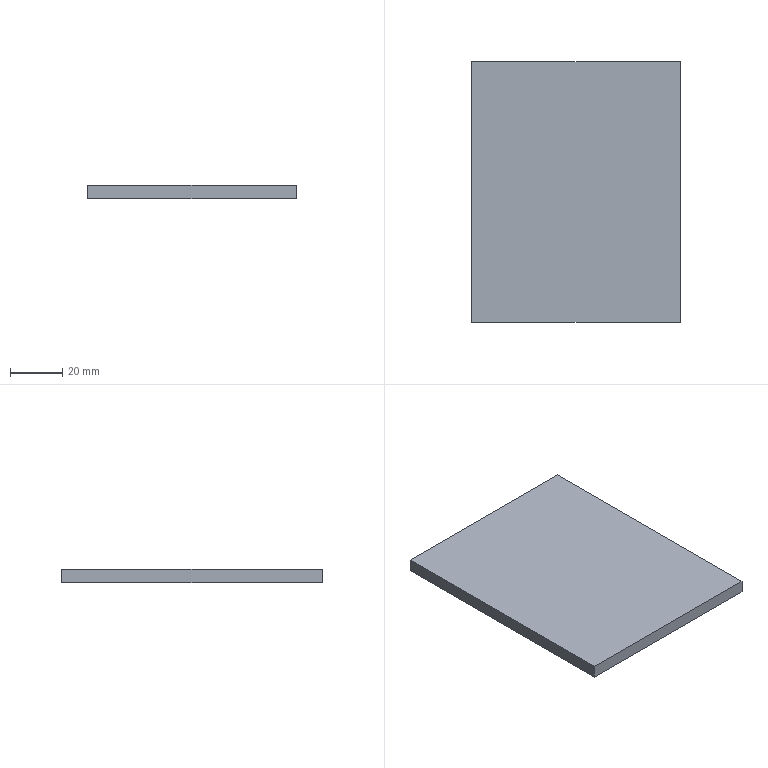Part | STEP file | MYT-A01-P41 | 1 solid | 6 faces | box 80 x 100 x 5 mm | volume 40000 mm3 | plane 6
STEP:
#1=CARTESIAN_POINT('',(40.,-50.,0.));
#2=VERTEX_POINT('',#1);
#3=CARTESIAN_POINT('',(40.,50.,0.));
#4=VERTEX_POINT('',#3);
#5=CARTESIAN_POINT('',(40.,50.,0.));
#6=DIRECTION('',(0.,1.,0.));
#7=VECTOR('',#6,1000.);
#8=LINE('',#5,#7);
#9=EDGE_CURVE('',#2,#4,#8,.T.);
#10=ORIENTED_EDGE('',*,*,#9,.T.);
#11=CARTESIAN_POINT('',(40.,50.,5.));
#12=VERTEX_POINT('',#11);
#13=CARTESIAN_POINT('',(40.,50.,5.));
#14=DIRECTION('',(0.,0.,-1.));
#15=VECTOR('',#14,1000.);
#16=LINE('',#13,#15);
#17=EDGE_CURVE('',#12,#4,#16,.T.);
#18=ORIENTED_EDGE('',*,*,#17,.F.);
#19=CARTESIAN_POINT('',(40.,-50.,5.));
#20=VERTEX_POINT('',#19);
#21=CARTESIAN_POINT('',(40.,50.,5.));
#22=DIRECTION('',(0.,1.,0.));
#23=VECTOR('',#22,1000.);
#24=LINE('',#21,#23);
#25=EDGE_CURVE('',#20,#12,#24,.T.);
#26=ORIENTED_EDGE('',*,*,#25,.F.);
#27=CARTESIAN_POINT('',(40.,-50.,5.));
#28=DIRECTION('',(0.,0.,-1.));
#29=VECTOR('',#28,1000.);
#30=LINE('',#27,#29);
#31=EDGE_CURVE('',#20,#2,#30,.T.);
#32=ORIENTED_EDGE('',*,*,#31,.T.);
#33=EDGE_LOOP('',(#10,#18,#26,#32));
#34=FACE_OUTER_BOUND('',#33,.T.);
#35=CARTESIAN_POINT('',(40.,50.,5.));
#36=DIRECTION('',(-1.,0.,0.));
#37=DIRECTION('',(0.,-1.,0.));
#38=AXIS2_PLACEMENT_3D('',#35,#36,#37);
#39=PLANE('',#38);
#40=ADVANCED_FACE('',(#34),#39,.F.);
#41=CARTESIAN_POINT('',(-40.,50.,0.));
#42=VERTEX_POINT('',#41);
#43=CARTESIAN_POINT('',(-40.,50.,0.));
#44=DIRECTION('',(-1.,0.,0.));
#45=VECTOR('',#44,1000.);
#46=LINE('',#43,#45);
#47=EDGE_CURVE('',#4,#42,#46,.T.);
#48=ORIENTED_EDGE('',*,*,#47,.T.);
#49=CARTESIAN_POINT('',(-40.,50.,5.));
#50=VERTEX_POINT('',#49);
#51=CARTESIAN_POINT('',(-40.,50.,5.));
#52=DIRECTION('',(0.,0.,-1.));
#53=VECTOR('',#52,1000.);
#54=LINE('',#51,#53);
#55=EDGE_CURVE('',#50,#42,#54,.T.);
#56=ORIENTED_EDGE('',*,*,#55,.F.);
#57=CARTESIAN_POINT('',(-40.,50.,5.));
#58=DIRECTION('',(-1.,0.,0.));
#59=VECTOR('',#58,1000.);
#60=LINE('',#57,#59);
#61=EDGE_CURVE('',#12,#50,#60,.T.);
#62=ORIENTED_EDGE('',*,*,#61,.F.);
#63=ORIENTED_EDGE('',*,*,#17,.T.);
#64=EDGE_LOOP('',(#48,#56,#62,#63));
#65=FACE_OUTER_BOUND('',#64,.T.);
#66=CARTESIAN_POINT('',(-40.,50.,5.));
#67=DIRECTION('',(0.,-1.,0.));
#68=DIRECTION('',(0.,0.,-1.));
#69=AXIS2_PLACEMENT_3D('',#66,#67,#68);
#70=PLANE('',#69);
#71=ADVANCED_FACE('',(#65),#70,.F.);
#72=CARTESIAN_POINT('',(-40.,-50.,0.));
#73=VERTEX_POINT('',#72);
#74=CARTESIAN_POINT('',(-40.,50.,0.));
#75=DIRECTION('',(0.,-1.,0.));
#76=VECTOR('',#75,1000.);
#77=LINE('',#74,#76);
#78=EDGE_CURVE('',#42,#73,#77,.T.);
#79=ORIENTED_EDGE('',*,*,#78,.T.);
#80=CARTESIAN_POINT('',(-40.,-50.,5.));
#81=VERTEX_POINT('',#80);
#82=CARTESIAN_POINT('',(-40.,-50.,5.));
#83=DIRECTION('',(0.,0.,-1.));
#84=VECTOR('',#83,1000.);
#85=LINE('',#82,#84);
#86=EDGE_CURVE('',#81,#73,#85,.T.);
#87=ORIENTED_EDGE('',*,*,#86,.F.);
#88=CARTESIAN_POINT('',(-40.,50.,5.));
#89=DIRECTION('',(0.,-1.,0.));
#90=VECTOR('',#89,1000.);
#91=LINE('',#88,#90);
#92=EDGE_CURVE('',#50,#81,#91,.T.);
#93=ORIENTED_EDGE('',*,*,#92,.F.);
#94=ORIENTED_EDGE('',*,*,#55,.T.);
#95=EDGE_LOOP('',(#79,#87,#93,#94));
#96=FACE_OUTER_BOUND('',#95,.T.);
#97=CARTESIAN_POINT('',(-40.,50.,5.));
#98=DIRECTION('',(1.,0.,0.));
#99=DIRECTION('',(0.,1.,0.));
#100=AXIS2_PLACEMENT_3D('',#97,#98,#99);
#101=PLANE('',#100);
#102=ADVANCED_FACE('',(#96),#101,.F.);
#103=CARTESIAN_POINT('',(-40.,-50.,0.));
#104=DIRECTION('',(1.,0.,0.));
#105=VECTOR('',#104,1000.);
#106=LINE('',#103,#105);
#107=EDGE_CURVE('',#73,#2,#106,.T.);
#108=ORIENTED_EDGE('',*,*,#107,.T.);
#109=ORIENTED_EDGE('',*,*,#31,.F.);
#110=CARTESIAN_POINT('',(-40.,-50.,5.));
#111=DIRECTION('',(1.,0.,0.));
#112=VECTOR('',#111,1000.);
#113=LINE('',#110,#112);
#114=EDGE_CURVE('',#81,#20,#113,.T.);
#115=ORIENTED_EDGE('',*,*,#114,.F.);
#116=ORIENTED_EDGE('',*,*,#86,.T.);
#117=EDGE_LOOP('',(#108,#109,#115,#116));
#118=FACE_OUTER_BOUND('',#117,.T.);
#119=CARTESIAN_POINT('',(-40.,-50.,5.));
#120=DIRECTION('',(0.,1.,0.));
#121=DIRECTION('',(0.,0.,1.));
#122=AXIS2_PLACEMENT_3D('',#119,#120,#121);
#123=PLANE('',#122);
#124=ADVANCED_FACE('',(#118),#123,.F.);
#125=ORIENTED_EDGE('',*,*,#25,.T.);
#126=ORIENTED_EDGE('',*,*,#61,.T.);
#127=ORIENTED_EDGE('',*,*,#92,.T.);
#128=ORIENTED_EDGE('',*,*,#114,.T.);
#129=EDGE_LOOP('',(#125,#126,#127,#128));
#130=FACE_OUTER_BOUND('',#129,.T.);
#131=CARTESIAN_POINT('',(0.,0.,5.));
#132=DIRECTION('',(0.,0.,1.));
#133=DIRECTION('',(1.,0.,0.));
#134=AXIS2_PLACEMENT_3D('',#131,#132,#133);
#135=PLANE('',#134);
#136=ADVANCED_FACE('',(#130),#135,.T.);
#137=ORIENTED_EDGE('',*,*,#9,.F.);
#138=ORIENTED_EDGE('',*,*,#107,.F.);
#139=ORIENTED_EDGE('',*,*,#78,.F.);
#140=ORIENTED_EDGE('',*,*,#47,.F.);
#141=EDGE_LOOP('',(#137,#138,#139,#140));
#142=FACE_OUTER_BOUND('',#141,.T.);
#143=CARTESIAN_POINT('',(0.,0.,0.));
#144=DIRECTION('',(0.,0.,1.));
#145=DIRECTION('',(1.,0.,0.));
#146=AXIS2_PLACEMENT_3D('',#143,#144,#145);
#147=PLANE('',#146);
#148=ADVANCED_FACE('',(#142),#147,.F.);
#149=CLOSED_SHELL('',(#40,#71,#102,#124,#136,#148));
#150=MANIFOLD_SOLID_BREP('',#149);
#151=CARTESIAN_POINT('',(0.,0.,0.));
#152=DIRECTION('',(0.,0.,1.));
#153=DIRECTION('',(1.,0.,0.));
#154=AXIS2_PLACEMENT_3D('',#151,#152,#153);
#155=(LENGTH_UNIT()NAMED_UNIT(*)SI_UNIT(.MILLI.,.METRE.));
#156=UNCERTAINTY_MEASURE_WITH_UNIT(LENGTH_MEASURE(0.00001),#155,'','');
#157=(NAMED_UNIT(*)PLANE_ANGLE_UNIT()SI_UNIT($,.RADIAN.));
#158=(NAMED_UNIT(*)SI_UNIT($,.STERADIAN.)SOLID_ANGLE_UNIT());
#159=(GEOMETRIC_REPRESENTATION_CONTEXT(3)GLOBAL_UNCERTAINTY_ASSIGNED_CONTEXT((#156))GLOBAL_UNIT_ASSIGNED_CONTEXT((#155,#157,#158))REPRESENTATION_CONTEXT('',''));
#160=ADVANCED_BREP_SHAPE_REPRESENTATION('',(#150,#154),#159);